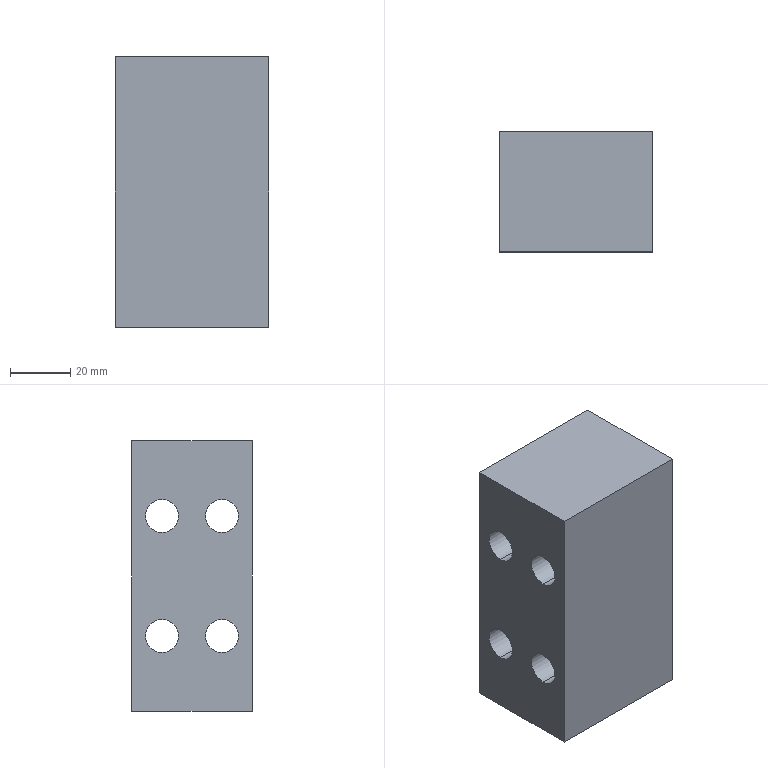Part | SolidWorks | features HoleWzd 2, Extrusion 1 | 1 solid | 34 faces | box 51 x 40 x 90 mm | volume 135826 mm3 | cylinder 20 | plane 10 | cone 4 | commonest cylinder face diameters 11 x8 18 x8 8.5 x4
STEP:
#1=CARTESIAN_POINT('',(26.5,0.,39.25));
#2=VERTEX_POINT('',#1);
#3=CARTESIAN_POINT('',(26.5,0.,30.75));
#4=VERTEX_POINT('',#3);
#5=CARTESIAN_POINT('',(26.5,0.,35.));
#6=DIRECTION('',(1.,0.,0.));
#7=DIRECTION('',(0.,0.,-1.));
#8=AXIS2_PLACEMENT_3D('',#5,#6,#7);
#9=CIRCLE('',#8,4.25);
#10=EDGE_CURVE('',#2,#4,#9,.T.);
#11=ORIENTED_EDGE('',*,*,#10,.F.);
#12=CARTESIAN_POINT('',(51.,0.,39.25));
#13=VERTEX_POINT('',#12);
#14=CARTESIAN_POINT('',(51.,0.,39.25));
#15=DIRECTION('',(1.,0.,0.));
#16=VECTOR('',#15,1000.);
#17=LINE('',#14,#16);
#18=EDGE_CURVE('',#2,#13,#17,.T.);
#19=ORIENTED_EDGE('',*,*,#18,.T.);
#20=CARTESIAN_POINT('',(51.,0.,30.75));
#21=VERTEX_POINT('',#20);
#22=CARTESIAN_POINT('',(51.,0.,35.));
#23=DIRECTION('',(1.,0.,0.));
#24=DIRECTION('',(0.,0.,-1.));
#25=AXIS2_PLACEMENT_3D('',#22,#23,#24);
#26=CIRCLE('',#25,4.25);
#27=EDGE_CURVE('',#13,#21,#26,.T.);
#28=ORIENTED_EDGE('',*,*,#27,.T.);
#29=CARTESIAN_POINT('',(51.,0.,30.75));
#30=DIRECTION('',(1.,0.,0.));
#31=VECTOR('',#30,1000.);
#32=LINE('',#29,#31);
#33=EDGE_CURVE('',#4,#21,#32,.T.);
#34=ORIENTED_EDGE('',*,*,#33,.F.);
#35=EDGE_LOOP('',(#11,#19,#28,#34));
#36=FACE_OUTER_BOUND('',#35,.T.);
#37=CARTESIAN_POINT('',(51.,0.,35.));
#38=DIRECTION('',(1.,0.,0.));
#39=DIRECTION('',(0.,0.,-1.));
#40=AXIS2_PLACEMENT_3D('',#37,#38,#39);
#41=CYLINDRICAL_SURFACE('',#40,4.25);
#42=ADVANCED_FACE('',(#36),#41,.F.);
#43=CARTESIAN_POINT('',(23.946,0.,35.));
#44=VERTEX_POINT('',#43);
#45=CARTESIAN_POINT('',(26.5,0.,30.75));
#46=DIRECTION('',(0.515,0.,-0.8572));
#47=VECTOR('',#46,1000.);
#48=LINE('',#45,#47);
#49=EDGE_CURVE('',#44,#4,#48,.T.);
#50=ORIENTED_EDGE('',*,*,#49,.F.);
#51=CARTESIAN_POINT('',(26.5,0.,39.25));
#52=DIRECTION('',(0.515,0.,0.8572));
#53=VECTOR('',#52,1000.);
#54=LINE('',#51,#53);
#55=EDGE_CURVE('',#44,#2,#54,.T.);
#56=ORIENTED_EDGE('',*,*,#55,.T.);
#57=ORIENTED_EDGE('',*,*,#10,.T.);
#58=EDGE_LOOP('',(#50,#56,#57));
#59=FACE_OUTER_BOUND('',#58,.T.);
#60=CARTESIAN_POINT('',(26.5,0.,35.));
#61=DIRECTION('',(1.,0.,0.));
#62=DIRECTION('',(0.,0.,-1.));
#63=AXIS2_PLACEMENT_3D('',#60,#61,#62);
#64=CONICAL_SURFACE('',#63,4.25,1.03);
#65=ADVANCED_FACE('',(#59),#64,.F.);
#66=CARTESIAN_POINT('',(26.5,0.,-30.75));
#67=VERTEX_POINT('',#66);
#68=CARTESIAN_POINT('',(26.5,0.,-39.25));
#69=VERTEX_POINT('',#68);
#70=CARTESIAN_POINT('',(26.5,0.,-35.));
#71=DIRECTION('',(1.,0.,0.));
#72=DIRECTION('',(0.,0.,-1.));
#73=AXIS2_PLACEMENT_3D('',#70,#71,#72);
#74=CIRCLE('',#73,4.25);
#75=EDGE_CURVE('',#67,#69,#74,.T.);
#76=ORIENTED_EDGE('',*,*,#75,.F.);
#77=CARTESIAN_POINT('',(51.,0.,-30.75));
#78=VERTEX_POINT('',#77);
#79=CARTESIAN_POINT('',(51.,0.,-30.75));
#80=DIRECTION('',(1.,0.,0.));
#81=VECTOR('',#80,1000.);
#82=LINE('',#79,#81);
#83=EDGE_CURVE('',#67,#78,#82,.T.);
#84=ORIENTED_EDGE('',*,*,#83,.T.);
#85=CARTESIAN_POINT('',(51.,0.,-39.25));
#86=VERTEX_POINT('',#85);
#87=CARTESIAN_POINT('',(51.,0.,-35.));
#88=DIRECTION('',(1.,0.,0.));
#89=DIRECTION('',(0.,0.,-1.));
#90=AXIS2_PLACEMENT_3D('',#87,#88,#89);
#91=CIRCLE('',#90,4.25);
#92=EDGE_CURVE('',#78,#86,#91,.T.);
#93=ORIENTED_EDGE('',*,*,#92,.T.);
#94=CARTESIAN_POINT('',(51.,0.,-39.25));
#95=DIRECTION('',(1.,0.,0.));
#96=VECTOR('',#95,1000.);
#97=LINE('',#94,#96);
#98=EDGE_CURVE('',#69,#86,#97,.T.);
#99=ORIENTED_EDGE('',*,*,#98,.F.);
#100=EDGE_LOOP('',(#76,#84,#93,#99));
#101=FACE_OUTER_BOUND('',#100,.T.);
#102=CARTESIAN_POINT('',(51.,0.,-35.));
#103=DIRECTION('',(1.,0.,0.));
#104=DIRECTION('',(0.,0.,-1.));
#105=AXIS2_PLACEMENT_3D('',#102,#103,#104);
#106=CYLINDRICAL_SURFACE('',#105,4.25);
#107=ADVANCED_FACE('',(#101),#106,.F.);
#108=CARTESIAN_POINT('',(23.946,0.,-35.));
#109=VERTEX_POINT('',#108);
#110=CARTESIAN_POINT('',(26.5,0.,-39.25));
#111=DIRECTION('',(0.515,0.,-0.8572));
#112=VECTOR('',#111,1000.);
#113=LINE('',#110,#112);
#114=EDGE_CURVE('',#109,#69,#113,.T.);
#115=ORIENTED_EDGE('',*,*,#114,.F.);
#116=CARTESIAN_POINT('',(26.5,0.,-30.75));
#117=DIRECTION('',(0.515,0.,0.8572));
#118=VECTOR('',#117,1000.);
#119=LINE('',#116,#118);
#120=EDGE_CURVE('',#109,#67,#119,.T.);
#121=ORIENTED_EDGE('',*,*,#120,.T.);
#122=ORIENTED_EDGE('',*,*,#75,.T.);
#123=EDGE_LOOP('',(#115,#121,#122));
#124=FACE_OUTER_BOUND('',#123,.T.);
#125=CARTESIAN_POINT('',(26.5,0.,-35.));
#126=DIRECTION('',(1.,0.,0.));
#127=DIRECTION('',(0.,0.,-1.));
#128=AXIS2_PLACEMENT_3D('',#125,#126,#127);
#129=CONICAL_SURFACE('',#128,4.25,1.03);
#130=ADVANCED_FACE('',(#124),#129,.F.);
#131=CARTESIAN_POINT('',(11.,10.,29.));
#132=VERTEX_POINT('',#131);
#133=CARTESIAN_POINT('',(11.,10.,11.));
#134=VERTEX_POINT('',#133);
#135=CARTESIAN_POINT('',(11.,10.,20.));
#136=DIRECTION('',(1.,0.,0.));
#137=DIRECTION('',(0.,0.,-1.));
#138=AXIS2_PLACEMENT_3D('',#135,#136,#137);
#139=CIRCLE('',#138,9.);
#140=EDGE_CURVE('',#132,#134,#139,.T.);
#141=ORIENTED_EDGE('',*,*,#140,.F.);
#142=CARTESIAN_POINT('',(51.,10.,29.));
#143=VERTEX_POINT('',#142);
#144=CARTESIAN_POINT('',(51.,10.,29.));
#145=DIRECTION('',(1.,0.,0.));
#146=VECTOR('',#145,1000.);
#147=LINE('',#144,#146);
#148=EDGE_CURVE('',#132,#143,#147,.T.);
#149=ORIENTED_EDGE('',*,*,#148,.T.);
#150=CARTESIAN_POINT('',(51.,10.,11.));
#151=VERTEX_POINT('',#150);
#152=CARTESIAN_POINT('',(51.,10.,20.));
#153=DIRECTION('',(1.,0.,0.));
#154=DIRECTION('',(0.,0.,-1.));
#155=AXIS2_PLACEMENT_3D('',#152,#153,#154);
#156=CIRCLE('',#155,9.);
#157=EDGE_CURVE('',#143,#151,#156,.T.);
#158=ORIENTED_EDGE('',*,*,#157,.T.);
#159=CARTESIAN_POINT('',(51.,10.,11.));
#160=DIRECTION('',(1.,0.,0.));
#161=VECTOR('',#160,1000.);
#162=LINE('',#159,#161);
#163=EDGE_CURVE('',#134,#151,#162,.T.);
#164=ORIENTED_EDGE('',*,*,#163,.F.);
#165=EDGE_LOOP('',(#141,#149,#158,#164));
#166=FACE_OUTER_BOUND('',#165,.T.);
#167=CARTESIAN_POINT('',(51.,10.,20.));
#168=DIRECTION('',(1.,0.,0.));
#169=DIRECTION('',(0.,0.,-1.));
#170=AXIS2_PLACEMENT_3D('',#167,#168,#169);
#171=CYLINDRICAL_SURFACE('',#170,9.);
#172=ADVANCED_FACE('',(#166),#171,.F.);
#173=CARTESIAN_POINT('',(0.,10.,25.5));
#174=VERTEX_POINT('',#173);
#175=CARTESIAN_POINT('',(0.,10.,14.5));
#176=VERTEX_POINT('',#175);
#177=CARTESIAN_POINT('',(0.,10.,20.));
#178=DIRECTION('',(1.,0.,0.));
#179=DIRECTION('',(0.,0.,-1.));
#180=AXIS2_PLACEMENT_3D('',#177,#178,#179);
#181=CIRCLE('',#180,5.5);
#182=EDGE_CURVE('',#174,#176,#181,.T.);
#183=ORIENTED_EDGE('',*,*,#182,.F.);
#184=CARTESIAN_POINT('',(11.,10.,25.5));
#185=VERTEX_POINT('',#184);
#186=CARTESIAN_POINT('',(51.,10.,25.5));
#187=DIRECTION('',(1.,0.,0.));
#188=VECTOR('',#187,1000.);
#189=LINE('',#186,#188);
#190=EDGE_CURVE('',#174,#185,#189,.T.);
#191=ORIENTED_EDGE('',*,*,#190,.T.);
#192=CARTESIAN_POINT('',(11.,10.,14.5));
#193=VERTEX_POINT('',#192);
#194=CARTESIAN_POINT('',(11.,10.,20.));
#195=DIRECTION('',(1.,0.,0.));
#196=DIRECTION('',(0.,0.,-1.));
#197=AXIS2_PLACEMENT_3D('',#194,#195,#196);
#198=CIRCLE('',#197,5.5);
#199=EDGE_CURVE('',#185,#193,#198,.T.);
#200=ORIENTED_EDGE('',*,*,#199,.T.);
#201=CARTESIAN_POINT('',(51.,10.,14.5));
#202=DIRECTION('',(1.,0.,0.));
#203=VECTOR('',#202,1000.);
#204=LINE('',#201,#203);
#205=EDGE_CURVE('',#176,#193,#204,.T.);
#206=ORIENTED_EDGE('',*,*,#205,.F.);
#207=EDGE_LOOP('',(#183,#191,#200,#206));
#208=FACE_OUTER_BOUND('',#207,.T.);
#209=CARTESIAN_POINT('',(51.,10.,20.));
#210=DIRECTION('',(1.,0.,0.));
#211=DIRECTION('',(0.,0.,-1.));
#212=AXIS2_PLACEMENT_3D('',#209,#210,#211);
#213=CYLINDRICAL_SURFACE('',#212,5.5);
#214=ADVANCED_FACE('',(#208),#213,.F.);
#215=CARTESIAN_POINT('',(11.,10.,-11.));
#216=VERTEX_POINT('',#215);
#217=CARTESIAN_POINT('',(11.,10.,-29.));
#218=VERTEX_POINT('',#217);
#219=CARTESIAN_POINT('',(11.,10.,-20.));
#220=DIRECTION('',(1.,0.,0.));
#221=DIRECTION('',(0.,0.,-1.));
#222=AXIS2_PLACEMENT_3D('',#219,#220,#221);
#223=CIRCLE('',#222,9.);
#224=EDGE_CURVE('',#216,#218,#223,.T.);
#225=ORIENTED_EDGE('',*,*,#224,.F.);
#226=CARTESIAN_POINT('',(51.,10.,-11.));
#227=VERTEX_POINT('',#226);
#228=CARTESIAN_POINT('',(51.,10.,-11.));
#229=DIRECTION('',(1.,0.,0.));
#230=VECTOR('',#229,1000.);
#231=LINE('',#228,#230);
#232=EDGE_CURVE('',#216,#227,#231,.T.);
#233=ORIENTED_EDGE('',*,*,#232,.T.);
#234=CARTESIAN_POINT('',(51.,10.,-29.));
#235=VERTEX_POINT('',#234);
#236=CARTESIAN_POINT('',(51.,10.,-20.));
#237=DIRECTION('',(1.,0.,0.));
#238=DIRECTION('',(0.,0.,-1.));
#239=AXIS2_PLACEMENT_3D('',#236,#237,#238);
#240=CIRCLE('',#239,9.);
#241=EDGE_CURVE('',#227,#235,#240,.T.);
#242=ORIENTED_EDGE('',*,*,#241,.T.);
#243=CARTESIAN_POINT('',(51.,10.,-29.));
#244=DIRECTION('',(1.,0.,0.));
#245=VECTOR('',#244,1000.);
#246=LINE('',#243,#245);
#247=EDGE_CURVE('',#218,#235,#246,.T.);
#248=ORIENTED_EDGE('',*,*,#247,.F.);
#249=EDGE_LOOP('',(#225,#233,#242,#248));
#250=FACE_OUTER_BOUND('',#249,.T.);
#251=CARTESIAN_POINT('',(51.,10.,-20.));
#252=DIRECTION('',(1.,0.,0.));
#253=DIRECTION('',(0.,0.,-1.));
#254=AXIS2_PLACEMENT_3D('',#251,#252,#253);
#255=CYLINDRICAL_SURFACE('',#254,9.);
#256=ADVANCED_FACE('',(#250),#255,.F.);
#257=CARTESIAN_POINT('',(0.,10.,-14.5));
#258=VERTEX_POINT('',#257);
#259=CARTESIAN_POINT('',(0.,10.,-25.5));
#260=VERTEX_POINT('',#259);
#261=CARTESIAN_POINT('',(0.,10.,-20.));
#262=DIRECTION('',(1.,0.,0.));
#263=DIRECTION('',(0.,0.,-1.));
#264=AXIS2_PLACEMENT_3D('',#261,#262,#263);
#265=CIRCLE('',#264,5.5);
#266=EDGE_CURVE('',#258,#260,#265,.T.);
#267=ORIENTED_EDGE('',*,*,#266,.F.);
#268=CARTESIAN_POINT('',(11.,10.,-14.5));
#269=VERTEX_POINT('',#268);
#270=CARTESIAN_POINT('',(51.,10.,-14.5));
#271=DIRECTION('',(1.,0.,0.));
#272=VECTOR('',#271,1000.);
#273=LINE('',#270,#272);
#274=EDGE_CURVE('',#258,#269,#273,.T.);
#275=ORIENTED_EDGE('',*,*,#274,.T.);
#276=CARTESIAN_POINT('',(11.,10.,-25.5));
#277=VERTEX_POINT('',#276);
#278=CARTESIAN_POINT('',(11.,10.,-20.));
#279=DIRECTION('',(1.,0.,0.));
#280=DIRECTION('',(0.,0.,-1.));
#281=AXIS2_PLACEMENT_3D('',#278,#279,#280);
#282=CIRCLE('',#281,5.5);
#283=EDGE_CURVE('',#269,#277,#282,.T.);
#284=ORIENTED_EDGE('',*,*,#283,.T.);
#285=CARTESIAN_POINT('',(51.,10.,-25.5));
#286=DIRECTION('',(1.,0.,0.));
#287=VECTOR('',#286,1000.);
#288=LINE('',#285,#287);
#289=EDGE_CURVE('',#260,#277,#288,.T.);
#290=ORIENTED_EDGE('',*,*,#289,.F.);
#291=EDGE_LOOP('',(#267,#275,#284,#290));
#292=FACE_OUTER_BOUND('',#291,.T.);
#293=CARTESIAN_POINT('',(51.,10.,-20.));
#294=DIRECTION('',(1.,0.,0.));
#295=DIRECTION('',(0.,0.,-1.));
#296=AXIS2_PLACEMENT_3D('',#293,#294,#295);
#297=CYLINDRICAL_SURFACE('',#296,5.5);
#298=ADVANCED_FACE('',(#292),#297,.F.);
#299=CARTESIAN_POINT('',(11.,-10.,29.));
#300=VERTEX_POINT('',#299);
#301=CARTESIAN_POINT('',(11.,-10.,11.));
#302=VERTEX_POINT('',#301);
#303=CARTESIAN_POINT('',(11.,-10.,20.));
#304=DIRECTION('',(1.,0.,0.));
#305=DIRECTION('',(0.,0.,-1.));
#306=AXIS2_PLACEMENT_3D('',#303,#304,#305);
#307=CIRCLE('',#306,9.);
#308=EDGE_CURVE('',#300,#302,#307,.T.);
#309=ORIENTED_EDGE('',*,*,#308,.F.);
#310=CARTESIAN_POINT('',(51.,-10.,29.));
#311=VERTEX_POINT('',#310);
#312=CARTESIAN_POINT('',(51.,-10.,29.));
#313=DIRECTION('',(1.,0.,0.));
#314=VECTOR('',#313,1000.);
#315=LINE('',#312,#314);
#316=EDGE_CURVE('',#300,#311,#315,.T.);
#317=ORIENTED_EDGE('',*,*,#316,.T.);
#318=CARTESIAN_POINT('',(51.,-10.,11.));
#319=VERTEX_POINT('',#318);
#320=CARTESIAN_POINT('',(51.,-10.,20.));
#321=DIRECTION('',(1.,0.,0.));
#322=DIRECTION('',(0.,0.,-1.));
#323=AXIS2_PLACEMENT_3D('',#320,#321,#322);
#324=CIRCLE('',#323,9.);
#325=EDGE_CURVE('',#311,#319,#324,.T.);
#326=ORIENTED_EDGE('',*,*,#325,.T.);
#327=CARTESIAN_POINT('',(51.,-10.,11.));
#328=DIRECTION('',(1.,0.,0.));
#329=VECTOR('',#328,1000.);
#330=LINE('',#327,#329);
#331=EDGE_CURVE('',#302,#319,#330,.T.);
#332=ORIENTED_EDGE('',*,*,#331,.F.);
#333=EDGE_LOOP('',(#309,#317,#326,#332));
#334=FACE_OUTER_BOUND('',#333,.T.);
#335=CARTESIAN_POINT('',(51.,-10.,20.));
#336=DIRECTION('',(1.,0.,0.));
#337=DIRECTION('',(0.,0.,-1.));
#338=AXIS2_PLACEMENT_3D('',#335,#336,#337);
#339=CYLINDRICAL_SURFACE('',#338,9.);
#340=ADVANCED_FACE('',(#334),#339,.F.);
#341=CARTESIAN_POINT('',(0.,-10.,25.5));
#342=VERTEX_POINT('',#341);
#343=CARTESIAN_POINT('',(0.,-10.,14.5));
#344=VERTEX_POINT('',#343);
#345=CARTESIAN_POINT('',(0.,-10.,20.));
#346=DIRECTION('',(1.,0.,0.));
#347=DIRECTION('',(0.,0.,-1.));
#348=AXIS2_PLACEMENT_3D('',#345,#346,#347);
#349=CIRCLE('',#348,5.5);
#350=EDGE_CURVE('',#342,#344,#349,.T.);
#351=ORIENTED_EDGE('',*,*,#350,.F.);
#352=CARTESIAN_POINT('',(11.,-10.,25.5));
#353=VERTEX_POINT('',#352);
#354=CARTESIAN_POINT('',(51.,-10.,25.5));
#355=DIRECTION('',(1.,0.,0.));
#356=VECTOR('',#355,1000.);
#357=LINE('',#354,#356);
#358=EDGE_CURVE('',#342,#353,#357,.T.);
#359=ORIENTED_EDGE('',*,*,#358,.T.);
#360=CARTESIAN_POINT('',(11.,-10.,14.5));
#361=VERTEX_POINT('',#360);
#362=CARTESIAN_POINT('',(11.,-10.,20.));
#363=DIRECTION('',(1.,0.,0.));
#364=DIRECTION('',(0.,0.,-1.));
#365=AXIS2_PLACEMENT_3D('',#362,#363,#364);
#366=CIRCLE('',#365,5.5);
#367=EDGE_CURVE('',#353,#361,#366,.T.);
#368=ORIENTED_EDGE('',*,*,#367,.T.);
#369=CARTESIAN_POINT('',(51.,-10.,14.5));
#370=DIRECTION('',(1.,0.,0.));
#371=VECTOR('',#370,1000.);
#372=LINE('',#369,#371);
#373=EDGE_CURVE('',#344,#361,#372,.T.);
#374=ORIENTED_EDGE('',*,*,#373,.F.);
#375=EDGE_LOOP('',(#351,#359,#368,#374));
#376=FACE_OUTER_BOUND('',#375,.T.);
#377=CARTESIAN_POINT('',(51.,-10.,20.));
#378=DIRECTION('',(1.,0.,0.));
#379=DIRECTION('',(0.,0.,-1.));
#380=AXIS2_PLACEMENT_3D('',#377,#378,#379);
#381=CYLINDRICAL_SURFACE('',#380,5.5);
#382=ADVANCED_FACE('',(#376),#381,.F.);
#383=CARTESIAN_POINT('',(11.,-10.,-11.));
#384=VERTEX_POINT('',#383);
#385=CARTESIAN_POINT('',(11.,-10.,-29.));
#386=VERTEX_POINT('',#385);
#387=CARTESIAN_POINT('',(11.,-10.,-20.));
#388=DIRECTION('',(1.,0.,0.));
#389=DIRECTION('',(0.,0.,-1.));
#390=AXIS2_PLACEMENT_3D('',#387,#388,#389);
#391=CIRCLE('',#390,9.);
#392=EDGE_CURVE('',#384,#386,#391,.T.);
#393=ORIENTED_EDGE('',*,*,#392,.F.);
#394=CARTESIAN_POINT('',(51.,-10.,-11.));
#395=VERTEX_POINT('',#394);
#396=CARTESIAN_POINT('',(51.,-10.,-11.));
#397=DIRECTION('',(1.,0.,0.));
#398=VECTOR('',#397,1000.);
#399=LINE('',#396,#398);
#400=EDGE_CURVE('',#384,#395,#399,.T.);
#401=ORIENTED_EDGE('',*,*,#400,.T.);
#402=CARTESIAN_POINT('',(51.,-10.,-29.));
#403=VERTEX_POINT('',#402);
#404=CARTESIAN_POINT('',(51.,-10.,-20.));
#405=DIRECTION('',(1.,0.,0.));
#406=DIRECTION('',(0.,0.,-1.));
#407=AXIS2_PLACEMENT_3D('',#404,#405,#406);
#408=CIRCLE('',#407,9.);
#409=EDGE_CURVE('',#395,#403,#408,.T.);
#410=ORIENTED_EDGE('',*,*,#409,.T.);
#411=CARTESIAN_POINT('',(51.,-10.,-29.));
#412=DIRECTION('',(1.,0.,0.));
#413=VECTOR('',#412,1000.);
#414=LINE('',#411,#413);
#415=EDGE_CURVE('',#386,#403,#414,.T.);
#416=ORIENTED_EDGE('',*,*,#415,.F.);
#417=EDGE_LOOP('',(#393,#401,#410,#416));
#418=FACE_OUTER_BOUND('',#417,.T.);
#419=CARTESIAN_POINT('',(51.,-10.,-20.));
#420=DIRECTION('',(1.,0.,0.));
#421=DIRECTION('',(0.,0.,-1.));
#422=AXIS2_PLACEMENT_3D('',#419,#420,#421);
#423=CYLINDRICAL_SURFACE('',#422,9.);
#424=ADVANCED_FACE('',(#418),#423,.F.);
#425=CARTESIAN_POINT('',(0.,-10.,-14.5));
#426=VERTEX_POINT('',#425);
#427=CARTESIAN_POINT('',(0.,-10.,-25.5));
#428=VERTEX_POINT('',#427);
#429=CARTESIAN_POINT('',(0.,-10.,-20.));
#430=DIRECTION('',(1.,0.,0.));
#431=DIRECTION('',(0.,0.,-1.));
#432=AXIS2_PLACEMENT_3D('',#429,#430,#431);
#433=CIRCLE('',#432,5.5);
#434=EDGE_CURVE('',#426,#428,#433,.T.);
#435=ORIENTED_EDGE('',*,*,#434,.F.);
#436=CARTESIAN_POINT('',(11.,-10.,-14.5));
#437=VERTEX_POINT('',#436);
#438=CARTESIAN_POINT('',(51.,-10.,-14.5));
#439=DIRECTION('',(1.,0.,0.));
#440=VECTOR('',#439,1000.);
#441=LINE('',#438,#440);
#442=EDGE_CURVE('',#426,#437,#441,.T.);
#443=ORIENTED_EDGE('',*,*,#442,.T.);
#444=CARTESIAN_POINT('',(11.,-10.,-25.5));
#445=VERTEX_POINT('',#444);
#446=CARTESIAN_POINT('',(11.,-10.,-20.));
#447=DIRECTION('',(1.,0.,0.));
#448=DIRECTION('',(0.,0.,-1.));
#449=AXIS2_PLACEMENT_3D('',#446,#447,#448);
#450=CIRCLE('',#449,5.5);
#451=EDGE_CURVE('',#437,#445,#450,.T.);
#452=ORIENTED_EDGE('',*,*,#451,.T.);
#453=CARTESIAN_POINT('',(51.,-10.,-25.5));
#454=DIRECTION('',(1.,0.,0.));
#455=VECTOR('',#454,1000.);
#456=LINE('',#453,#455);
#457=EDGE_CURVE('',#428,#445,#456,.T.);
#458=ORIENTED_EDGE('',*,*,#457,.F.);
#459=EDGE_LOOP('',(#435,#443,#452,#458));
#460=FACE_OUTER_BOUND('',#459,.T.);
#461=CARTESIAN_POINT('',(51.,-10.,-20.));
#462=DIRECTION('',(1.,0.,0.));
#463=DIRECTION('',(0.,0.,-1.));
#464=AXIS2_PLACEMENT_3D('',#461,#462,#463);
#465=CYLINDRICAL_SURFACE('',#464,5.5);
#466=ADVANCED_FACE('',(#460),#465,.F.);
#467=CARTESIAN_POINT('',(0.,-20.,-45.));
#468=VERTEX_POINT('',#467);
#469=CARTESIAN_POINT('',(0.,20.,-45.));
#470=VERTEX_POINT('',#469);
#471=CARTESIAN_POINT('',(0.,20.,-45.));
#472=DIRECTION('',(0.,1.,0.));
#473=VECTOR('',#472,1000.);
#474=LINE('',#471,#473);
#475=EDGE_CURVE('',#468,#470,#474,.T.);
#476=ORIENTED_EDGE('',*,*,#475,.T.);
#477=CARTESIAN_POINT('',(51.,20.,-45.));
#478=VERTEX_POINT('',#477);
#479=CARTESIAN_POINT('',(51.,20.,-45.));
#480=DIRECTION('',(-1.,0.,0.));
#481=VECTOR('',#480,1000.);
#482=LINE('',#479,#481);
#483=EDGE_CURVE('',#478,#470,#482,.T.);
#484=ORIENTED_EDGE('',*,*,#483,.F.);
#485=CARTESIAN_POINT('',(51.,-20.,-45.));
#486=VERTEX_POINT('',#485);
#487=CARTESIAN_POINT('',(51.,20.,-45.));
#488=DIRECTION('',(0.,1.,0.));
#489=VECTOR('',#488,1000.);
#490=LINE('',#487,#489);
#491=EDGE_CURVE('',#486,#478,#490,.T.);
#492=ORIENTED_EDGE('',*,*,#491,.F.);
#493=CARTESIAN_POINT('',(51.,-20.,-45.));
#494=DIRECTION('',(-1.,0.,0.));
#495=VECTOR('',#494,1000.);
#496=LINE('',#493,#495);
#497=EDGE_CURVE('',#486,#468,#496,.T.);
#498=ORIENTED_EDGE('',*,*,#497,.T.);
#499=EDGE_LOOP('',(#476,#484,#492,#498));
#500=FACE_OUTER_BOUND('',#499,.T.);
#501=CARTESIAN_POINT('',(51.,20.,-45.));
#502=DIRECTION('',(0.,0.,1.));
#503=DIRECTION('',(0.,-1.,0.));
#504=AXIS2_PLACEMENT_3D('',#501,#502,#503);
#505=PLANE('',#504);
#506=ADVANCED_FACE('',(#500),#505,.F.);
#507=CARTESIAN_POINT('',(0.,20.,45.));
#508=VERTEX_POINT('',#507);
#509=CARTESIAN_POINT('',(0.,20.,45.));
#510=DIRECTION('',(0.,0.,1.));
#511=VECTOR('',#510,1000.);
#512=LINE('',#509,#511);
#513=EDGE_CURVE('',#470,#508,#512,.T.);
#514=ORIENTED_EDGE('',*,*,#513,.T.);
#515=CARTESIAN_POINT('',(51.,20.,45.));
#516=VERTEX_POINT('',#515);
#517=CARTESIAN_POINT('',(51.,20.,45.));
#518=DIRECTION('',(-1.,0.,0.));
#519=VECTOR('',#518,1000.);
#520=LINE('',#517,#519);
#521=EDGE_CURVE('',#516,#508,#520,.T.);
#522=ORIENTED_EDGE('',*,*,#521,.F.);
#523=CARTESIAN_POINT('',(51.,20.,45.));
#524=DIRECTION('',(0.,0.,1.));
#525=VECTOR('',#524,1000.);
#526=LINE('',#523,#525);
#527=EDGE_CURVE('',#478,#516,#526,.T.);
#528=ORIENTED_EDGE('',*,*,#527,.F.);
#529=ORIENTED_EDGE('',*,*,#483,.T.);
#530=EDGE_LOOP('',(#514,#522,#528,#529));
#531=FACE_OUTER_BOUND('',#530,.T.);
#532=CARTESIAN_POINT('',(51.,20.,45.));
#533=DIRECTION('',(0.,-1.,0.));
#534=DIRECTION('',(0.,0.,-1.));
#535=AXIS2_PLACEMENT_3D('',#532,#533,#534);
#536=PLANE('',#535);
#537=ADVANCED_FACE('',(#531),#536,.F.);
#538=CARTESIAN_POINT('',(0.,-20.,45.));
#539=VERTEX_POINT('',#538);
#540=CARTESIAN_POINT('',(0.,20.,45.));
#541=DIRECTION('',(0.,-1.,0.));
#542=VECTOR('',#541,1000.);
#543=LINE('',#540,#542);
#544=EDGE_CURVE('',#508,#539,#543,.T.);
#545=ORIENTED_EDGE('',*,*,#544,.T.);
#546=CARTESIAN_POINT('',(51.,-20.,45.));
#547=VERTEX_POINT('',#546);
#548=CARTESIAN_POINT('',(51.,-20.,45.));
#549=DIRECTION('',(-1.,0.,0.));
#550=VECTOR('',#549,1000.);
#551=LINE('',#548,#550);
#552=EDGE_CURVE('',#547,#539,#551,.T.);
#553=ORIENTED_EDGE('',*,*,#552,.F.);
#554=CARTESIAN_POINT('',(51.,20.,45.));
#555=DIRECTION('',(0.,-1.,0.));
#556=VECTOR('',#555,1000.);
#557=LINE('',#554,#556);
#558=EDGE_CURVE('',#516,#547,#557,.T.);
#559=ORIENTED_EDGE('',*,*,#558,.F.);
#560=ORIENTED_EDGE('',*,*,#521,.T.);
#561=EDGE_LOOP('',(#545,#553,#559,#560));
#562=FACE_OUTER_BOUND('',#561,.T.);
#563=CARTESIAN_POINT('',(51.,20.,45.));
#564=DIRECTION('',(0.,0.,-1.));
#565=DIRECTION('',(0.,1.,0.));
#566=AXIS2_PLACEMENT_3D('',#563,#564,#565);
#567=PLANE('',#566);
#568=ADVANCED_FACE('',(#562),#567,.F.);
#569=CARTESIAN_POINT('',(0.,-20.,45.));
#570=DIRECTION('',(0.,0.,-1.));
#571=VECTOR('',#570,1000.);
#572=LINE('',#569,#571);
#573=EDGE_CURVE('',#539,#468,#572,.T.);
#574=ORIENTED_EDGE('',*,*,#573,.T.);
#575=ORIENTED_EDGE('',*,*,#497,.F.);
#576=CARTESIAN_POINT('',(51.,-20.,45.));
#577=DIRECTION('',(0.,0.,-1.));
#578=VECTOR('',#577,1000.);
#579=LINE('',#576,#578);
#580=EDGE_CURVE('',#547,#486,#579,.T.);
#581=ORIENTED_EDGE('',*,*,#580,.F.);
#582=ORIENTED_EDGE('',*,*,#552,.T.);
#583=EDGE_LOOP('',(#574,#575,#581,#582));
#584=FACE_OUTER_BOUND('',#583,.T.);
#585=CARTESIAN_POINT('',(51.,-20.,45.));
#586=DIRECTION('',(0.,1.,0.));
#587=DIRECTION('',(0.,0.,1.));
#588=AXIS2_PLACEMENT_3D('',#585,#586,#587);
#589=PLANE('',#588);
#590=ADVANCED_FACE('',(#584),#589,.F.);
#591=CARTESIAN_POINT('',(51.,0.,35.));
#592=DIRECTION('',(1.,0.,0.));
#593=DIRECTION('',(0.,0.,-1.));
#594=AXIS2_PLACEMENT_3D('',#591,#592,#593);
#595=CIRCLE('',#594,4.25);
#596=EDGE_CURVE('',#21,#13,#595,.T.);
#597=ORIENTED_EDGE('',*,*,#596,.F.);
#598=ORIENTED_EDGE('',*,*,#27,.F.);
#599=EDGE_LOOP('',(#597,#598));
#600=FACE_BOUND('',#599,.T.);
#601=CARTESIAN_POINT('',(51.,0.,-35.));
#602=DIRECTION('',(1.,0.,0.));
#603=DIRECTION('',(0.,0.,-1.));
#604=AXIS2_PLACEMENT_3D('',#601,#602,#603);
#605=CIRCLE('',#604,4.25);
#606=EDGE_CURVE('',#86,#78,#605,.T.);
#607=ORIENTED_EDGE('',*,*,#606,.F.);
#608=ORIENTED_EDGE('',*,*,#92,.F.);
#609=EDGE_LOOP('',(#607,#608));
#610=FACE_BOUND('',#609,.T.);
#611=CARTESIAN_POINT('',(51.,10.,20.));
#612=DIRECTION('',(1.,0.,0.));
#613=DIRECTION('',(0.,0.,-1.));
#614=AXIS2_PLACEMENT_3D('',#611,#612,#613);
#615=CIRCLE('',#614,9.);
#616=EDGE_CURVE('',#151,#143,#615,.T.);
#617=ORIENTED_EDGE('',*,*,#616,.F.);
#618=ORIENTED_EDGE('',*,*,#157,.F.);
#619=EDGE_LOOP('',(#617,#618));
#620=FACE_BOUND('',#619,.T.);
#621=CARTESIAN_POINT('',(51.,10.,-20.));
#622=DIRECTION('',(1.,0.,0.));
#623=DIRECTION('',(0.,0.,-1.));
#624=AXIS2_PLACEMENT_3D('',#621,#622,#623);
#625=CIRCLE('',#624,9.);
#626=EDGE_CURVE('',#235,#227,#625,.T.);
#627=ORIENTED_EDGE('',*,*,#626,.F.);
#628=ORIENTED_EDGE('',*,*,#241,.F.);
#629=EDGE_LOOP('',(#627,#628));
#630=FACE_BOUND('',#629,.T.);
#631=CARTESIAN_POINT('',(51.,-10.,20.));
#632=DIRECTION('',(1.,0.,0.));
#633=DIRECTION('',(0.,0.,-1.));
#634=AXIS2_PLACEMENT_3D('',#631,#632,#633);
#635=CIRCLE('',#634,9.);
#636=EDGE_CURVE('',#319,#311,#635,.T.);
#637=ORIENTED_EDGE('',*,*,#636,.F.);
#638=ORIENTED_EDGE('',*,*,#325,.F.);
#639=EDGE_LOOP('',(#637,#638));
#640=FACE_BOUND('',#639,.T.);
#641=CARTESIAN_POINT('',(51.,-10.,-20.));
#642=DIRECTION('',(1.,0.,0.));
#643=DIRECTION('',(0.,0.,-1.));
#644=AXIS2_PLACEMENT_3D('',#641,#642,#643);
#645=CIRCLE('',#644,9.);
#646=EDGE_CURVE('',#403,#395,#645,.T.);
#647=ORIENTED_EDGE('',*,*,#646,.F.);
#648=ORIENTED_EDGE('',*,*,#409,.F.);
#649=EDGE_LOOP('',(#647,#648));
#650=FACE_BOUND('',#649,.T.);
#651=ORIENTED_EDGE('',*,*,#491,.T.);
#652=ORIENTED_EDGE('',*,*,#527,.T.);
#653=ORIENTED_EDGE('',*,*,#558,.T.);
#654=ORIENTED_EDGE('',*,*,#580,.T.);
#655=EDGE_LOOP('',(#651,#652,#653,#654));
#656=FACE_OUTER_BOUND('',#655,.T.);
#657=CARTESIAN_POINT('',(51.,0.,0.));
#658=DIRECTION('',(1.,0.,0.));
#659=DIRECTION('',(0.,0.,-1.));
#660=AXIS2_PLACEMENT_3D('',#657,#658,#659);
#661=PLANE('',#660);
#662=ADVANCED_FACE('',(#600,#610,#620,#630,#640,#650,#656),#661,.T.);
#663=CARTESIAN_POINT('',(0.,10.,20.));
#664=DIRECTION('',(1.,0.,0.));
#665=DIRECTION('',(0.,0.,-1.));
#666=AXIS2_PLACEMENT_3D('',#663,#664,#665);
#667=CIRCLE('',#666,5.5);
#668=EDGE_CURVE('',#176,#174,#667,.T.);
#669=ORIENTED_EDGE('',*,*,#668,.T.);
#670=ORIENTED_EDGE('',*,*,#182,.T.);
#671=EDGE_LOOP('',(#669,#670));
#672=FACE_BOUND('',#671,.T.);
#673=CARTESIAN_POINT('',(0.,10.,-20.));
#674=DIRECTION('',(1.,0.,0.));
#675=DIRECTION('',(0.,0.,-1.));
#676=AXIS2_PLACEMENT_3D('',#673,#674,#675);
#677=CIRCLE('',#676,5.5);
#678=EDGE_CURVE('',#260,#258,#677,.T.);
#679=ORIENTED_EDGE('',*,*,#678,.T.);
#680=ORIENTED_EDGE('',*,*,#266,.T.);
#681=EDGE_LOOP('',(#679,#680));
#682=FACE_BOUND('',#681,.T.);
#683=CARTESIAN_POINT('',(0.,-10.,20.));
#684=DIRECTION('',(1.,0.,0.));
#685=DIRECTION('',(0.,0.,-1.));
#686=AXIS2_PLACEMENT_3D('',#683,#684,#685);
#687=CIRCLE('',#686,5.5);
#688=EDGE_CURVE('',#344,#342,#687,.T.);
#689=ORIENTED_EDGE('',*,*,#688,.T.);
#690=ORIENTED_EDGE('',*,*,#350,.T.);
#691=EDGE_LOOP('',(#689,#690));
#692=FACE_BOUND('',#691,.T.);
#693=CARTESIAN_POINT('',(0.,-10.,-20.));
#694=DIRECTION('',(1.,0.,0.));
#695=DIRECTION('',(0.,0.,-1.));
#696=AXIS2_PLACEMENT_3D('',#693,#694,#695);
#697=CIRCLE('',#696,5.5);
#698=EDGE_CURVE('',#428,#426,#697,.T.);
#699=ORIENTED_EDGE('',*,*,#698,.T.);
#700=ORIENTED_EDGE('',*,*,#434,.T.);
#701=EDGE_LOOP('',(#699,#700));
#702=FACE_BOUND('',#701,.T.);
#703=ORIENTED_EDGE('',*,*,#475,.F.);
#704=ORIENTED_EDGE('',*,*,#573,.F.);
#705=ORIENTED_EDGE('',*,*,#544,.F.);
#706=ORIENTED_EDGE('',*,*,#513,.F.);
#707=EDGE_LOOP('',(#703,#704,#705,#706));
#708=FACE_OUTER_BOUND('',#707,.T.);
#709=CARTESIAN_POINT('',(0.,0.,0.));
#710=DIRECTION('',(1.,0.,0.));
#711=DIRECTION('',(0.,0.,-1.));
#712=AXIS2_PLACEMENT_3D('',#709,#710,#711);
#713=PLANE('',#712);
#714=ADVANCED_FACE('',(#672,#682,#692,#702,#708),#713,.F.);
#715=ORIENTED_EDGE('',*,*,#442,.F.);
#716=ORIENTED_EDGE('',*,*,#698,.F.);
#717=ORIENTED_EDGE('',*,*,#457,.T.);
#718=CARTESIAN_POINT('',(11.,-10.,-20.));
#719=DIRECTION('',(1.,0.,0.));
#720=DIRECTION('',(0.,0.,-1.));
#721=AXIS2_PLACEMENT_3D('',#718,#719,#720);
#722=CIRCLE('',#721,5.5);
#723=EDGE_CURVE('',#445,#437,#722,.T.);
#724=ORIENTED_EDGE('',*,*,#723,.T.);
#725=EDGE_LOOP('',(#715,#716,#717,#724));
#726=FACE_OUTER_BOUND('',#725,.T.);
#727=CARTESIAN_POINT('',(51.,-10.,-20.));
#728=DIRECTION('',(1.,0.,0.));
#729=DIRECTION('',(0.,0.,-1.));
#730=AXIS2_PLACEMENT_3D('',#727,#728,#729);
#731=CYLINDRICAL_SURFACE('',#730,5.5);
#732=ADVANCED_FACE('',(#726),#731,.F.);
#733=ORIENTED_EDGE('',*,*,#723,.F.);
#734=ORIENTED_EDGE('',*,*,#451,.F.);
#735=EDGE_LOOP('',(#733,#734));
#736=FACE_BOUND('',#735,.T.);
#737=CARTESIAN_POINT('',(11.,-10.,-20.));
#738=DIRECTION('',(1.,0.,0.));
#739=DIRECTION('',(0.,0.,-1.));
#740=AXIS2_PLACEMENT_3D('',#737,#738,#739);
#741=CIRCLE('',#740,9.);
#742=EDGE_CURVE('',#386,#384,#741,.T.);
#743=ORIENTED_EDGE('',*,*,#742,.T.);
#744=ORIENTED_EDGE('',*,*,#392,.T.);
#745=EDGE_LOOP('',(#743,#744));
#746=FACE_OUTER_BOUND('',#745,.T.);
#747=CARTESIAN_POINT('',(11.,-4.5,-20.));
#748=DIRECTION('',(-1.,0.,0.));
#749=DIRECTION('',(0.,0.,1.));
#750=AXIS2_PLACEMENT_3D('',#747,#748,#749);
#751=PLANE('',#750);
#752=ADVANCED_FACE('',(#736,#746),#751,.F.);
#753=ORIENTED_EDGE('',*,*,#400,.F.);
#754=ORIENTED_EDGE('',*,*,#742,.F.);
#755=ORIENTED_EDGE('',*,*,#415,.T.);
#756=ORIENTED_EDGE('',*,*,#646,.T.);
#757=EDGE_LOOP('',(#753,#754,#755,#756));
#758=FACE_OUTER_BOUND('',#757,.T.);
#759=CARTESIAN_POINT('',(51.,-10.,-20.));
#760=DIRECTION('',(1.,0.,0.));
#761=DIRECTION('',(0.,0.,-1.));
#762=AXIS2_PLACEMENT_3D('',#759,#760,#761);
#763=CYLINDRICAL_SURFACE('',#762,9.);
#764=ADVANCED_FACE('',(#758),#763,.F.);
#765=ORIENTED_EDGE('',*,*,#358,.F.);
#766=ORIENTED_EDGE('',*,*,#688,.F.);
#767=ORIENTED_EDGE('',*,*,#373,.T.);
#768=CARTESIAN_POINT('',(11.,-10.,20.));
#769=DIRECTION('',(1.,0.,0.));
#770=DIRECTION('',(0.,0.,-1.));
#771=AXIS2_PLACEMENT_3D('',#768,#769,#770);
#772=CIRCLE('',#771,5.5);
#773=EDGE_CURVE('',#361,#353,#772,.T.);
#774=ORIENTED_EDGE('',*,*,#773,.T.);
#775=EDGE_LOOP('',(#765,#766,#767,#774));
#776=FACE_OUTER_BOUND('',#775,.T.);
#777=CARTESIAN_POINT('',(51.,-10.,20.));
#778=DIRECTION('',(1.,0.,0.));
#779=DIRECTION('',(0.,0.,-1.));
#780=AXIS2_PLACEMENT_3D('',#777,#778,#779);
#781=CYLINDRICAL_SURFACE('',#780,5.5);
#782=ADVANCED_FACE('',(#776),#781,.F.);
#783=ORIENTED_EDGE('',*,*,#773,.F.);
#784=ORIENTED_EDGE('',*,*,#367,.F.);
#785=EDGE_LOOP('',(#783,#784));
#786=FACE_BOUND('',#785,.T.);
#787=CARTESIAN_POINT('',(11.,-10.,20.));
#788=DIRECTION('',(1.,0.,0.));
#789=DIRECTION('',(0.,0.,-1.));
#790=AXIS2_PLACEMENT_3D('',#787,#788,#789);
#791=CIRCLE('',#790,9.);
#792=EDGE_CURVE('',#302,#300,#791,.T.);
#793=ORIENTED_EDGE('',*,*,#792,.T.);
#794=ORIENTED_EDGE('',*,*,#308,.T.);
#795=EDGE_LOOP('',(#793,#794));
#796=FACE_OUTER_BOUND('',#795,.T.);
#797=CARTESIAN_POINT('',(11.,-4.5,20.));
#798=DIRECTION('',(-1.,0.,0.));
#799=DIRECTION('',(0.,0.,1.));
#800=AXIS2_PLACEMENT_3D('',#797,#798,#799);
#801=PLANE('',#800);
#802=ADVANCED_FACE('',(#786,#796),#801,.F.);
#803=ORIENTED_EDGE('',*,*,#316,.F.);
#804=ORIENTED_EDGE('',*,*,#792,.F.);
#805=ORIENTED_EDGE('',*,*,#331,.T.);
#806=ORIENTED_EDGE('',*,*,#636,.T.);
#807=EDGE_LOOP('',(#803,#804,#805,#806));
#808=FACE_OUTER_BOUND('',#807,.T.);
#809=CARTESIAN_POINT('',(51.,-10.,20.));
#810=DIRECTION('',(1.,0.,0.));
#811=DIRECTION('',(0.,0.,-1.));
#812=AXIS2_PLACEMENT_3D('',#809,#810,#811);
#813=CYLINDRICAL_SURFACE('',#812,9.);
#814=ADVANCED_FACE('',(#808),#813,.F.);
#815=ORIENTED_EDGE('',*,*,#274,.F.);
#816=ORIENTED_EDGE('',*,*,#678,.F.);
#817=ORIENTED_EDGE('',*,*,#289,.T.);
#818=CARTESIAN_POINT('',(11.,10.,-20.));
#819=DIRECTION('',(1.,0.,0.));
#820=DIRECTION('',(0.,0.,-1.));
#821=AXIS2_PLACEMENT_3D('',#818,#819,#820);
#822=CIRCLE('',#821,5.5);
#823=EDGE_CURVE('',#277,#269,#822,.T.);
#824=ORIENTED_EDGE('',*,*,#823,.T.);
#825=EDGE_LOOP('',(#815,#816,#817,#824));
#826=FACE_OUTER_BOUND('',#825,.T.);
#827=CARTESIAN_POINT('',(51.,10.,-20.));
#828=DIRECTION('',(1.,0.,0.));
#829=DIRECTION('',(0.,0.,-1.));
#830=AXIS2_PLACEMENT_3D('',#827,#828,#829);
#831=CYLINDRICAL_SURFACE('',#830,5.5);
#832=ADVANCED_FACE('',(#826),#831,.F.);
#833=ORIENTED_EDGE('',*,*,#823,.F.);
#834=ORIENTED_EDGE('',*,*,#283,.F.);
#835=EDGE_LOOP('',(#833,#834));
#836=FACE_BOUND('',#835,.T.);
#837=CARTESIAN_POINT('',(11.,10.,-20.));
#838=DIRECTION('',(1.,0.,0.));
#839=DIRECTION('',(0.,0.,-1.));
#840=AXIS2_PLACEMENT_3D('',#837,#838,#839);
#841=CIRCLE('',#840,9.);
#842=EDGE_CURVE('',#218,#216,#841,.T.);
#843=ORIENTED_EDGE('',*,*,#842,.T.);
#844=ORIENTED_EDGE('',*,*,#224,.T.);
#845=EDGE_LOOP('',(#843,#844));
#846=FACE_OUTER_BOUND('',#845,.T.);
#847=CARTESIAN_POINT('',(11.,15.5,-20.));
#848=DIRECTION('',(-1.,0.,0.));
#849=DIRECTION('',(0.,0.,1.));
#850=AXIS2_PLACEMENT_3D('',#847,#848,#849);
#851=PLANE('',#850);
#852=ADVANCED_FACE('',(#836,#846),#851,.F.);
#853=ORIENTED_EDGE('',*,*,#232,.F.);
#854=ORIENTED_EDGE('',*,*,#842,.F.);
#855=ORIENTED_EDGE('',*,*,#247,.T.);
#856=ORIENTED_EDGE('',*,*,#626,.T.);
#857=EDGE_LOOP('',(#853,#854,#855,#856));
#858=FACE_OUTER_BOUND('',#857,.T.);
#859=CARTESIAN_POINT('',(51.,10.,-20.));
#860=DIRECTION('',(1.,0.,0.));
#861=DIRECTION('',(0.,0.,-1.));
#862=AXIS2_PLACEMENT_3D('',#859,#860,#861);
#863=CYLINDRICAL_SURFACE('',#862,9.);
#864=ADVANCED_FACE('',(#858),#863,.F.);
#865=ORIENTED_EDGE('',*,*,#190,.F.);
#866=ORIENTED_EDGE('',*,*,#668,.F.);
#867=ORIENTED_EDGE('',*,*,#205,.T.);
#868=CARTESIAN_POINT('',(11.,10.,20.));
#869=DIRECTION('',(1.,0.,0.));
#870=DIRECTION('',(0.,0.,-1.));
#871=AXIS2_PLACEMENT_3D('',#868,#869,#870);
#872=CIRCLE('',#871,5.5);
#873=EDGE_CURVE('',#193,#185,#872,.T.);
#874=ORIENTED_EDGE('',*,*,#873,.T.);
#875=EDGE_LOOP('',(#865,#866,#867,#874));
#876=FACE_OUTER_BOUND('',#875,.T.);
#877=CARTESIAN_POINT('',(51.,10.,20.));
#878=DIRECTION('',(1.,0.,0.));
#879=DIRECTION('',(0.,0.,-1.));
#880=AXIS2_PLACEMENT_3D('',#877,#878,#879);
#881=CYLINDRICAL_SURFACE('',#880,5.5);
#882=ADVANCED_FACE('',(#876),#881,.F.);
#883=ORIENTED_EDGE('',*,*,#873,.F.);
#884=ORIENTED_EDGE('',*,*,#199,.F.);
#885=EDGE_LOOP('',(#883,#884));
#886=FACE_BOUND('',#885,.T.);
#887=CARTESIAN_POINT('',(11.,10.,20.));
#888=DIRECTION('',(1.,0.,0.));
#889=DIRECTION('',(0.,0.,-1.));
#890=AXIS2_PLACEMENT_3D('',#887,#888,#889);
#891=CIRCLE('',#890,9.);
#892=EDGE_CURVE('',#134,#132,#891,.T.);
#893=ORIENTED_EDGE('',*,*,#892,.T.);
#894=ORIENTED_EDGE('',*,*,#140,.T.);
#895=EDGE_LOOP('',(#893,#894));
#896=FACE_OUTER_BOUND('',#895,.T.);
#897=CARTESIAN_POINT('',(11.,15.5,20.));
#898=DIRECTION('',(-1.,0.,0.));
#899=DIRECTION('',(0.,0.,1.));
#900=AXIS2_PLACEMENT_3D('',#897,#898,#899);
#901=PLANE('',#900);
#902=ADVANCED_FACE('',(#886,#896),#901,.F.);
#903=ORIENTED_EDGE('',*,*,#148,.F.);
#904=ORIENTED_EDGE('',*,*,#892,.F.);
#905=ORIENTED_EDGE('',*,*,#163,.T.);
#906=ORIENTED_EDGE('',*,*,#616,.T.);
#907=EDGE_LOOP('',(#903,#904,#905,#906));
#908=FACE_OUTER_BOUND('',#907,.T.);
#909=CARTESIAN_POINT('',(51.,10.,20.));
#910=DIRECTION('',(1.,0.,0.));
#911=DIRECTION('',(0.,0.,-1.));
#912=AXIS2_PLACEMENT_3D('',#909,#910,#911);
#913=CYLINDRICAL_SURFACE('',#912,9.);
#914=ADVANCED_FACE('',(#908),#913,.F.);
#915=ORIENTED_EDGE('',*,*,#120,.F.);
#916=ORIENTED_EDGE('',*,*,#114,.T.);
#917=CARTESIAN_POINT('',(26.5,0.,-35.));
#918=DIRECTION('',(1.,0.,0.));
#919=DIRECTION('',(0.,0.,-1.));
#920=AXIS2_PLACEMENT_3D('',#917,#918,#919);
#921=CIRCLE('',#920,4.25);
#922=EDGE_CURVE('',#69,#67,#921,.T.);
#923=ORIENTED_EDGE('',*,*,#922,.T.);
#924=EDGE_LOOP('',(#915,#916,#923));
#925=FACE_OUTER_BOUND('',#924,.T.);
#926=CARTESIAN_POINT('',(26.5,0.,-35.));
#927=DIRECTION('',(1.,0.,0.));
#928=DIRECTION('',(0.,0.,-1.));
#929=AXIS2_PLACEMENT_3D('',#926,#927,#928);
#930=CONICAL_SURFACE('',#929,4.25,1.03);
#931=ADVANCED_FACE('',(#925),#930,.F.);
#932=ORIENTED_EDGE('',*,*,#83,.F.);
#933=ORIENTED_EDGE('',*,*,#922,.F.);
#934=ORIENTED_EDGE('',*,*,#98,.T.);
#935=ORIENTED_EDGE('',*,*,#606,.T.);
#936=EDGE_LOOP('',(#932,#933,#934,#935));
#937=FACE_OUTER_BOUND('',#936,.T.);
#938=CARTESIAN_POINT('',(51.,0.,-35.));
#939=DIRECTION('',(1.,0.,0.));
#940=DIRECTION('',(0.,0.,-1.));
#941=AXIS2_PLACEMENT_3D('',#938,#939,#940);
#942=CYLINDRICAL_SURFACE('',#941,4.25);
#943=ADVANCED_FACE('',(#937),#942,.F.);
#944=ORIENTED_EDGE('',*,*,#55,.F.);
#945=ORIENTED_EDGE('',*,*,#49,.T.);
#946=CARTESIAN_POINT('',(26.5,0.,35.));
#947=DIRECTION('',(1.,0.,0.));
#948=DIRECTION('',(0.,0.,-1.));
#949=AXIS2_PLACEMENT_3D('',#946,#947,#948);
#950=CIRCLE('',#949,4.25);
#951=EDGE_CURVE('',#4,#2,#950,.T.);
#952=ORIENTED_EDGE('',*,*,#951,.T.);
#953=EDGE_LOOP('',(#944,#945,#952));
#954=FACE_OUTER_BOUND('',#953,.T.);
#955=CARTESIAN_POINT('',(26.5,0.,35.));
#956=DIRECTION('',(1.,0.,0.));
#957=DIRECTION('',(0.,0.,-1.));
#958=AXIS2_PLACEMENT_3D('',#955,#956,#957);
#959=CONICAL_SURFACE('',#958,4.25,1.03);
#960=ADVANCED_FACE('',(#954),#959,.F.);
#961=ORIENTED_EDGE('',*,*,#18,.F.);
#962=ORIENTED_EDGE('',*,*,#951,.F.);
#963=ORIENTED_EDGE('',*,*,#33,.T.);
#964=ORIENTED_EDGE('',*,*,#596,.T.);
#965=EDGE_LOOP('',(#961,#962,#963,#964));
#966=FACE_OUTER_BOUND('',#965,.T.);
#967=CARTESIAN_POINT('',(51.,0.,35.));
#968=DIRECTION('',(1.,0.,0.));
#969=DIRECTION('',(0.,0.,-1.));
#970=AXIS2_PLACEMENT_3D('',#967,#968,#969);
#971=CYLINDRICAL_SURFACE('',#970,4.25);
#972=ADVANCED_FACE('',(#966),#971,.F.);
#973=CLOSED_SHELL('',(#42,#65,#107,#130,#172,#214,#256,#298,#340,#382,#424,#466,#506,#537,#568,#590,#662,#714,#732,#752,#764,#782,#802,#814,#832,#852,#864,#882,#902,#914,#931,#943,#960,#972));
#974=MANIFOLD_SOLID_BREP('',#973);
#975=CARTESIAN_POINT('',(0.,0.,0.));
#976=DIRECTION('',(0.,0.,1.));
#977=DIRECTION('',(1.,0.,0.));
#978=AXIS2_PLACEMENT_3D('',#975,#976,#977);
#979=(LENGTH_UNIT()NAMED_UNIT(*)SI_UNIT(.MILLI.,.METRE.));
#980=UNCERTAINTY_MEASURE_WITH_UNIT(LENGTH_MEASURE(0.00001),#979,'','');
#981=(NAMED_UNIT(*)PLANE_ANGLE_UNIT()SI_UNIT($,.RADIAN.));
#982=(NAMED_UNIT(*)SI_UNIT($,.STERADIAN.)SOLID_ANGLE_UNIT());
#983=(GEOMETRIC_REPRESENTATION_CONTEXT(3)GLOBAL_UNCERTAINTY_ASSIGNED_CONTEXT((#980))GLOBAL_UNIT_ASSIGNED_CONTEXT((#979,#981,#982))REPRESENTATION_CONTEXT('',''));
#984=ADVANCED_BREP_SHAPE_REPRESENTATION('',(#974,#978),#983);